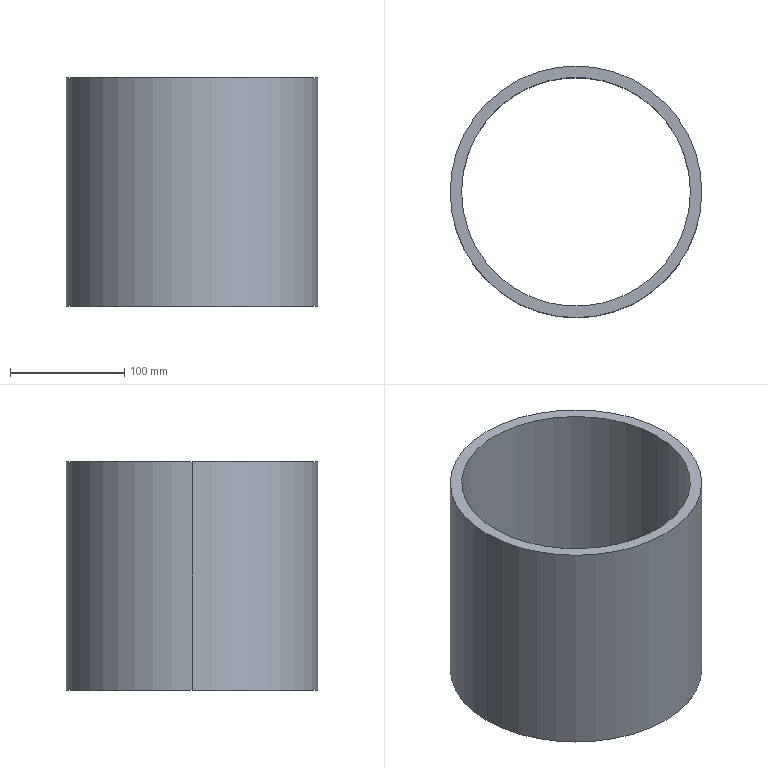Part | SolidWorks | features ExtruThin 1 | 1 solid | 6 faces | box 220 x 220 x 200 mm | volume 1319469 mm3 | cylinder 4 | plane 2 | commonest cylinder face diameters 200 x2 220 x2
STEP:
#1=CARTESIAN_POINT('',(-100.,0.,200.));
#2=VERTEX_POINT('',#1);
#3=CARTESIAN_POINT('',(100.,0.,200.));
#4=VERTEX_POINT('',#3);
#5=CARTESIAN_POINT('',(0.,0.,200.));
#6=DIRECTION('',(0.,0.,1.));
#7=DIRECTION('',(1.,0.,0.));
#8=AXIS2_PLACEMENT_3D('',#5,#6,#7);
#9=CIRCLE('',#8,100.);
#10=EDGE_CURVE('',#2,#4,#9,.T.);
#11=ORIENTED_EDGE('',*,*,#10,.T.);
#12=CARTESIAN_POINT('',(100.,0.,0.));
#13=VERTEX_POINT('',#12);
#14=CARTESIAN_POINT('',(100.,0.,200.));
#15=DIRECTION('',(0.,0.,-1.));
#16=VECTOR('',#15,1000.);
#17=LINE('',#14,#16);
#18=EDGE_CURVE('',#4,#13,#17,.T.);
#19=ORIENTED_EDGE('',*,*,#18,.T.);
#20=CARTESIAN_POINT('',(-100.,0.,0.));
#21=VERTEX_POINT('',#20);
#22=CARTESIAN_POINT('',(0.,0.,0.));
#23=DIRECTION('',(0.,0.,1.));
#24=DIRECTION('',(1.,0.,0.));
#25=AXIS2_PLACEMENT_3D('',#22,#23,#24);
#26=CIRCLE('',#25,100.);
#27=EDGE_CURVE('',#21,#13,#26,.T.);
#28=ORIENTED_EDGE('',*,*,#27,.F.);
#29=CARTESIAN_POINT('',(-100.,0.,200.));
#30=DIRECTION('',(0.,0.,-1.));
#31=VECTOR('',#30,1000.);
#32=LINE('',#29,#31);
#33=EDGE_CURVE('',#2,#21,#32,.T.);
#34=ORIENTED_EDGE('',*,*,#33,.F.);
#35=EDGE_LOOP('',(#11,#19,#28,#34));
#36=FACE_OUTER_BOUND('',#35,.T.);
#37=CARTESIAN_POINT('',(0.,0.,200.));
#38=DIRECTION('',(0.,0.,-1.));
#39=DIRECTION('',(-1.,0.,0.));
#40=AXIS2_PLACEMENT_3D('',#37,#38,#39);
#41=CYLINDRICAL_SURFACE('',#40,100.);
#42=ADVANCED_FACE('',(#36),#41,.F.);
#43=CARTESIAN_POINT('',(110.,0.,200.));
#44=VERTEX_POINT('',#43);
#45=CARTESIAN_POINT('',(-110.,0.,200.));
#46=VERTEX_POINT('',#45);
#47=CARTESIAN_POINT('',(0.,0.,200.));
#48=DIRECTION('',(0.,0.,1.));
#49=DIRECTION('',(1.,0.,0.));
#50=AXIS2_PLACEMENT_3D('',#47,#48,#49);
#51=CIRCLE('',#50,110.);
#52=EDGE_CURVE('',#44,#46,#51,.T.);
#53=ORIENTED_EDGE('',*,*,#52,.F.);
#54=CARTESIAN_POINT('',(110.,0.,0.));
#55=VERTEX_POINT('',#54);
#56=CARTESIAN_POINT('',(110.,0.,200.));
#57=DIRECTION('',(0.,0.,-1.));
#58=VECTOR('',#57,1000.);
#59=LINE('',#56,#58);
#60=EDGE_CURVE('',#44,#55,#59,.T.);
#61=ORIENTED_EDGE('',*,*,#60,.T.);
#62=CARTESIAN_POINT('',(-110.,0.,0.));
#63=VERTEX_POINT('',#62);
#64=CARTESIAN_POINT('',(0.,0.,0.));
#65=DIRECTION('',(0.,0.,1.));
#66=DIRECTION('',(1.,0.,0.));
#67=AXIS2_PLACEMENT_3D('',#64,#65,#66);
#68=CIRCLE('',#67,110.);
#69=EDGE_CURVE('',#55,#63,#68,.T.);
#70=ORIENTED_EDGE('',*,*,#69,.T.);
#71=CARTESIAN_POINT('',(-110.,0.,200.));
#72=DIRECTION('',(0.,0.,-1.));
#73=VECTOR('',#72,1000.);
#74=LINE('',#71,#73);
#75=EDGE_CURVE('',#46,#63,#74,.T.);
#76=ORIENTED_EDGE('',*,*,#75,.F.);
#77=EDGE_LOOP('',(#53,#61,#70,#76));
#78=FACE_OUTER_BOUND('',#77,.T.);
#79=CARTESIAN_POINT('',(0.,0.,200.));
#80=DIRECTION('',(0.,0.,-1.));
#81=DIRECTION('',(-1.,0.,0.));
#82=AXIS2_PLACEMENT_3D('',#79,#80,#81);
#83=CYLINDRICAL_SURFACE('',#82,110.);
#84=ADVANCED_FACE('',(#78),#83,.T.);
#85=CARTESIAN_POINT('',(0.,0.,200.));
#86=DIRECTION('',(0.,0.,1.));
#87=DIRECTION('',(1.,0.,0.));
#88=AXIS2_PLACEMENT_3D('',#85,#86,#87);
#89=CIRCLE('',#88,110.);
#90=EDGE_CURVE('',#46,#44,#89,.T.);
#91=ORIENTED_EDGE('',*,*,#90,.T.);
#92=ORIENTED_EDGE('',*,*,#52,.T.);
#93=EDGE_LOOP('',(#91,#92));
#94=FACE_OUTER_BOUND('',#93,.T.);
#95=ORIENTED_EDGE('',*,*,#10,.F.);
#96=CARTESIAN_POINT('',(0.,0.,200.));
#97=DIRECTION('',(0.,0.,1.));
#98=DIRECTION('',(1.,0.,0.));
#99=AXIS2_PLACEMENT_3D('',#96,#97,#98);
#100=CIRCLE('',#99,100.);
#101=EDGE_CURVE('',#4,#2,#100,.T.);
#102=ORIENTED_EDGE('',*,*,#101,.F.);
#103=EDGE_LOOP('',(#95,#102));
#104=FACE_BOUND('',#103,.T.);
#105=CARTESIAN_POINT('',(0.,0.,200.));
#106=DIRECTION('',(0.,0.,1.));
#107=DIRECTION('',(1.,0.,0.));
#108=AXIS2_PLACEMENT_3D('',#105,#106,#107);
#109=PLANE('',#108);
#110=ADVANCED_FACE('',(#94,#104),#109,.T.);
#111=CARTESIAN_POINT('',(0.,0.,0.));
#112=DIRECTION('',(0.,0.,1.));
#113=DIRECTION('',(1.,0.,0.));
#114=AXIS2_PLACEMENT_3D('',#111,#112,#113);
#115=CIRCLE('',#114,110.);
#116=EDGE_CURVE('',#63,#55,#115,.T.);
#117=ORIENTED_EDGE('',*,*,#116,.F.);
#118=ORIENTED_EDGE('',*,*,#69,.F.);
#119=EDGE_LOOP('',(#117,#118));
#120=FACE_OUTER_BOUND('',#119,.T.);
#121=ORIENTED_EDGE('',*,*,#27,.T.);
#122=CARTESIAN_POINT('',(0.,0.,0.));
#123=DIRECTION('',(0.,0.,1.));
#124=DIRECTION('',(1.,0.,0.));
#125=AXIS2_PLACEMENT_3D('',#122,#123,#124);
#126=CIRCLE('',#125,100.);
#127=EDGE_CURVE('',#13,#21,#126,.T.);
#128=ORIENTED_EDGE('',*,*,#127,.T.);
#129=EDGE_LOOP('',(#121,#128));
#130=FACE_BOUND('',#129,.T.);
#131=CARTESIAN_POINT('',(0.,0.,0.));
#132=DIRECTION('',(0.,0.,1.));
#133=DIRECTION('',(1.,0.,0.));
#134=AXIS2_PLACEMENT_3D('',#131,#132,#133);
#135=PLANE('',#134);
#136=ADVANCED_FACE('',(#120,#130),#135,.F.);
#137=ORIENTED_EDGE('',*,*,#60,.F.);
#138=ORIENTED_EDGE('',*,*,#90,.F.);
#139=ORIENTED_EDGE('',*,*,#75,.T.);
#140=ORIENTED_EDGE('',*,*,#116,.T.);
#141=EDGE_LOOP('',(#137,#138,#139,#140));
#142=FACE_OUTER_BOUND('',#141,.T.);
#143=CARTESIAN_POINT('',(0.,0.,200.));
#144=DIRECTION('',(0.,0.,-1.));
#145=DIRECTION('',(-1.,0.,0.));
#146=AXIS2_PLACEMENT_3D('',#143,#144,#145);
#147=CYLINDRICAL_SURFACE('',#146,110.);
#148=ADVANCED_FACE('',(#142),#147,.T.);
#149=ORIENTED_EDGE('',*,*,#18,.F.);
#150=ORIENTED_EDGE('',*,*,#101,.T.);
#151=ORIENTED_EDGE('',*,*,#33,.T.);
#152=ORIENTED_EDGE('',*,*,#127,.F.);
#153=EDGE_LOOP('',(#149,#150,#151,#152));
#154=FACE_OUTER_BOUND('',#153,.T.);
#155=CARTESIAN_POINT('',(0.,0.,200.));
#156=DIRECTION('',(0.,0.,-1.));
#157=DIRECTION('',(-1.,0.,0.));
#158=AXIS2_PLACEMENT_3D('',#155,#156,#157);
#159=CYLINDRICAL_SURFACE('',#158,100.);
#160=ADVANCED_FACE('',(#154),#159,.F.);
#161=CLOSED_SHELL('',(#42,#84,#110,#136,#148,#160));
#162=MANIFOLD_SOLID_BREP('',#161);
#163=CARTESIAN_POINT('',(0.,0.,0.));
#164=DIRECTION('',(0.,0.,1.));
#165=DIRECTION('',(1.,0.,0.));
#166=AXIS2_PLACEMENT_3D('',#163,#164,#165);
#167=(LENGTH_UNIT()NAMED_UNIT(*)SI_UNIT(.MILLI.,.METRE.));
#168=UNCERTAINTY_MEASURE_WITH_UNIT(LENGTH_MEASURE(0.00001),#167,'','');
#169=(NAMED_UNIT(*)PLANE_ANGLE_UNIT()SI_UNIT($,.RADIAN.));
#170=(NAMED_UNIT(*)SI_UNIT($,.STERADIAN.)SOLID_ANGLE_UNIT());
#171=(GEOMETRIC_REPRESENTATION_CONTEXT(3)GLOBAL_UNCERTAINTY_ASSIGNED_CONTEXT((#168))GLOBAL_UNIT_ASSIGNED_CONTEXT((#167,#169,#170))REPRESENTATION_CONTEXT('',''));
#172=ADVANCED_BREP_SHAPE_REPRESENTATION('',(#162,#166),#171);